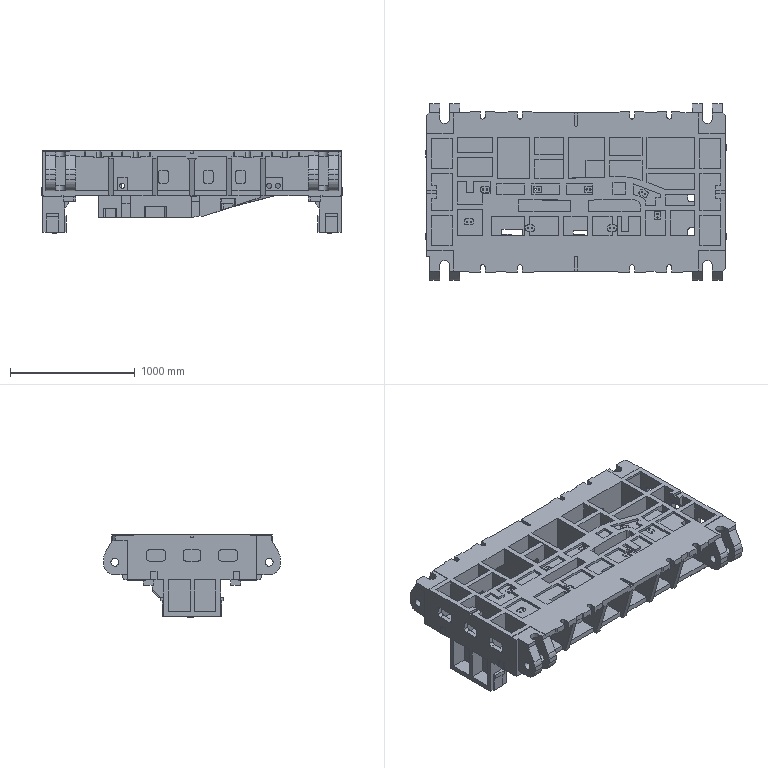Part | NX | features solid 2 | 1 solid | 1277 faces | box 2410 x 1420 x 660 mm | volume 490263198 mm3 | plane 1007 | cylinder 236 | spline 34 | commonest cylinder face diameters 30 x80 40 x73 80 x22 11.5 x16 180 x16 63.5 x8